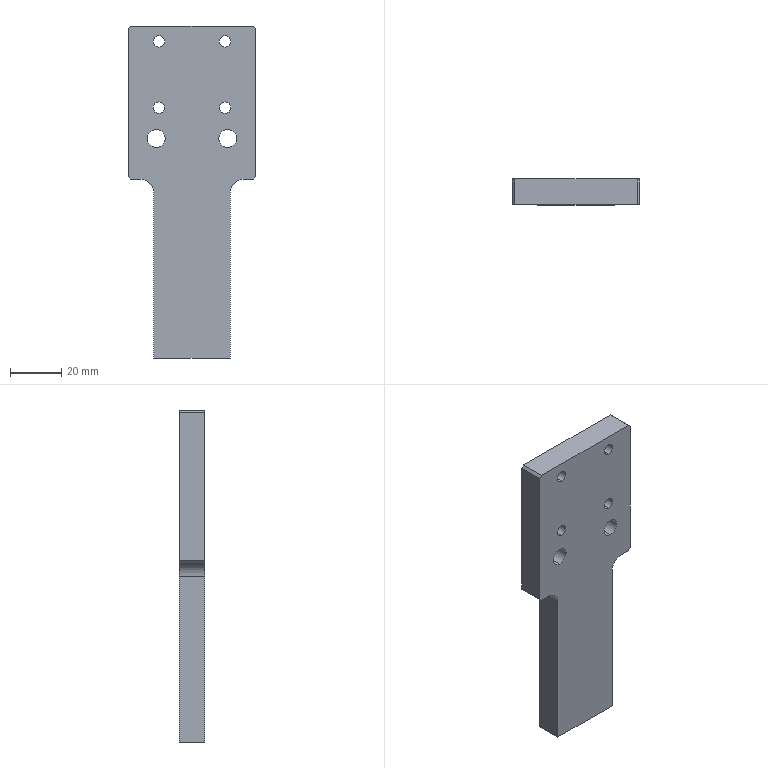Part | 1 solid | 48 faces | box 50 x 10 x 130 mm | volume 48871 mm3 | cylinder 26 | plane 18 | cone 4 | commonest cylinder face diameters 4.5 x8 8 x8 3.3 x4 7 x4 10 x2
STEP:
#1=CARTESIAN_POINT('',(-8.35,0.,-89.9));
#2=VERTEX_POINT('',#1);
#3=CARTESIAN_POINT('',(-11.65,0.,-89.9));
#4=VERTEX_POINT('',#3);
#5=CARTESIAN_POINT('',(-10.,0.,-89.9));
#6=DIRECTION('',(0.,0.,-1.));
#7=DIRECTION('',(-1.,0.,0.));
#8=AXIS2_PLACEMENT_3D('',#5,#6,#7);
#9=CIRCLE('',#8,1.65);
#10=EDGE_CURVE('',#2,#4,#9,.T.);
#11=ORIENTED_EDGE('',*,*,#10,.F.);
#12=CARTESIAN_POINT('',(-8.35,0.,-100.));
#13=VERTEX_POINT('',#12);
#14=CARTESIAN_POINT('',(-8.35,0.,-100.));
#15=DIRECTION('',(0.,0.,-1.));
#16=VECTOR('',#15,1000.);
#17=LINE('',#14,#16);
#18=EDGE_CURVE('',#2,#13,#17,.T.);
#19=ORIENTED_EDGE('',*,*,#18,.T.);
#20=CARTESIAN_POINT('',(-11.65,0.,-100.));
#21=VERTEX_POINT('',#20);
#22=CARTESIAN_POINT('',(-10.,0.,-100.));
#23=DIRECTION('',(0.,0.,-1.));
#24=DIRECTION('',(-1.,0.,0.));
#25=AXIS2_PLACEMENT_3D('',#22,#23,#24);
#26=CIRCLE('',#25,1.65);
#27=EDGE_CURVE('',#13,#21,#26,.T.);
#28=ORIENTED_EDGE('',*,*,#27,.T.);
#29=CARTESIAN_POINT('',(-11.65,0.,-100.));
#30=DIRECTION('',(0.,0.,-1.));
#31=VECTOR('',#30,1000.);
#32=LINE('',#29,#31);
#33=EDGE_CURVE('',#4,#21,#32,.T.);
#34=ORIENTED_EDGE('',*,*,#33,.F.);
#35=EDGE_LOOP('',(#11,#19,#28,#34));
#36=FACE_OUTER_BOUND('',#35,.T.);
#37=CARTESIAN_POINT('',(-10.,0.,-100.));
#38=DIRECTION('',(0.,0.,-1.));
#39=DIRECTION('',(-1.,0.,0.));
#40=AXIS2_PLACEMENT_3D('',#37,#38,#39);
#41=CYLINDRICAL_SURFACE('',#40,1.65);
#42=ADVANCED_FACE('',(#36),#41,.F.);
#43=CARTESIAN_POINT('',(-10.,0.,-88.909));
#44=VERTEX_POINT('',#43);
#45=CARTESIAN_POINT('',(-11.65,0.,-89.9));
#46=DIRECTION('',(-0.8572,0.,-0.515));
#47=VECTOR('',#46,1000.);
#48=LINE('',#45,#47);
#49=EDGE_CURVE('',#44,#4,#48,.T.);
#50=ORIENTED_EDGE('',*,*,#49,.F.);
#51=CARTESIAN_POINT('',(-8.35,0.,-89.9));
#52=DIRECTION('',(0.8572,0.,-0.515));
#53=VECTOR('',#52,1000.);
#54=LINE('',#51,#53);
#55=EDGE_CURVE('',#44,#2,#54,.T.);
#56=ORIENTED_EDGE('',*,*,#55,.T.);
#57=ORIENTED_EDGE('',*,*,#10,.T.);
#58=EDGE_LOOP('',(#50,#56,#57));
#59=FACE_OUTER_BOUND('',#58,.T.);
#60=CARTESIAN_POINT('',(-10.,0.,-89.9));
#61=DIRECTION('',(0.,0.,-1.));
#62=DIRECTION('',(-1.,0.,0.));
#63=AXIS2_PLACEMENT_3D('',#60,#61,#62);
#64=CONICAL_SURFACE('',#63,1.65,1.03);
#65=ADVANCED_FACE('',(#59),#64,.F.);
#66=CARTESIAN_POINT('',(11.65,0.,-89.9));
#67=VERTEX_POINT('',#66);
#68=CARTESIAN_POINT('',(8.35,0.,-89.9));
#69=VERTEX_POINT('',#68);
#70=CARTESIAN_POINT('',(10.,0.,-89.9));
#71=DIRECTION('',(0.,0.,-1.));
#72=DIRECTION('',(-1.,0.,0.));
#73=AXIS2_PLACEMENT_3D('',#70,#71,#72);
#74=CIRCLE('',#73,1.65);
#75=EDGE_CURVE('',#67,#69,#74,.T.);
#76=ORIENTED_EDGE('',*,*,#75,.F.);
#77=CARTESIAN_POINT('',(11.65,0.,-100.));
#78=VERTEX_POINT('',#77);
#79=CARTESIAN_POINT('',(11.65,0.,-100.));
#80=DIRECTION('',(0.,0.,-1.));
#81=VECTOR('',#80,1000.);
#82=LINE('',#79,#81);
#83=EDGE_CURVE('',#67,#78,#82,.T.);
#84=ORIENTED_EDGE('',*,*,#83,.T.);
#85=CARTESIAN_POINT('',(8.35,0.,-100.));
#86=VERTEX_POINT('',#85);
#87=CARTESIAN_POINT('',(10.,0.,-100.));
#88=DIRECTION('',(0.,0.,-1.));
#89=DIRECTION('',(-1.,0.,0.));
#90=AXIS2_PLACEMENT_3D('',#87,#88,#89);
#91=CIRCLE('',#90,1.65);
#92=EDGE_CURVE('',#78,#86,#91,.T.);
#93=ORIENTED_EDGE('',*,*,#92,.T.);
#94=CARTESIAN_POINT('',(8.35,0.,-100.));
#95=DIRECTION('',(0.,0.,-1.));
#96=VECTOR('',#95,1000.);
#97=LINE('',#94,#96);
#98=EDGE_CURVE('',#69,#86,#97,.T.);
#99=ORIENTED_EDGE('',*,*,#98,.F.);
#100=EDGE_LOOP('',(#76,#84,#93,#99));
#101=FACE_OUTER_BOUND('',#100,.T.);
#102=CARTESIAN_POINT('',(10.,0.,-100.));
#103=DIRECTION('',(0.,0.,-1.));
#104=DIRECTION('',(-1.,0.,0.));
#105=AXIS2_PLACEMENT_3D('',#102,#103,#104);
#106=CYLINDRICAL_SURFACE('',#105,1.65);
#107=ADVANCED_FACE('',(#101),#106,.F.);
#108=CARTESIAN_POINT('',(10.,0.,-88.909));
#109=VERTEX_POINT('',#108);
#110=CARTESIAN_POINT('',(8.35,0.,-89.9));
#111=DIRECTION('',(-0.8572,0.,-0.515));
#112=VECTOR('',#111,1000.);
#113=LINE('',#110,#112);
#114=EDGE_CURVE('',#109,#69,#113,.T.);
#115=ORIENTED_EDGE('',*,*,#114,.F.);
#116=CARTESIAN_POINT('',(11.65,0.,-89.9));
#117=DIRECTION('',(0.8572,0.,-0.515));
#118=VECTOR('',#117,1000.);
#119=LINE('',#116,#118);
#120=EDGE_CURVE('',#109,#67,#119,.T.);
#121=ORIENTED_EDGE('',*,*,#120,.T.);
#122=ORIENTED_EDGE('',*,*,#75,.T.);
#123=EDGE_LOOP('',(#115,#121,#122));
#124=FACE_OUTER_BOUND('',#123,.T.);
#125=CARTESIAN_POINT('',(10.,0.,-89.9));
#126=DIRECTION('',(0.,0.,-1.));
#127=DIRECTION('',(-1.,0.,0.));
#128=AXIS2_PLACEMENT_3D('',#125,#126,#127);
#129=CONICAL_SURFACE('',#128,1.65,1.03);
#130=ADVANCED_FACE('',(#124),#129,.F.);
#131=CARTESIAN_POINT('',(-14.,-5.,-17.5));
#132=VERTEX_POINT('',#131);
#133=CARTESIAN_POINT('',(-14.,-5.,-10.5));
#134=VERTEX_POINT('',#133);
#135=CARTESIAN_POINT('',(-14.,-5.,-14.));
#136=DIRECTION('',(0.,1.,0.));
#137=DIRECTION('',(0.,0.,1.));
#138=AXIS2_PLACEMENT_3D('',#135,#136,#137);
#139=CIRCLE('',#138,3.5);
#140=EDGE_CURVE('',#132,#134,#139,.T.);
#141=ORIENTED_EDGE('',*,*,#140,.F.);
#142=CARTESIAN_POINT('',(-14.,5.,-17.5));
#143=VERTEX_POINT('',#142);
#144=CARTESIAN_POINT('',(-14.,5.,-17.5));
#145=DIRECTION('',(0.,1.,0.));
#146=VECTOR('',#145,1000.);
#147=LINE('',#144,#146);
#148=EDGE_CURVE('',#132,#143,#147,.T.);
#149=ORIENTED_EDGE('',*,*,#148,.T.);
#150=CARTESIAN_POINT('',(-14.,5.,-10.5));
#151=VERTEX_POINT('',#150);
#152=CARTESIAN_POINT('',(-14.,5.,-14.));
#153=DIRECTION('',(0.,1.,0.));
#154=DIRECTION('',(0.,0.,1.));
#155=AXIS2_PLACEMENT_3D('',#152,#153,#154);
#156=CIRCLE('',#155,3.5);
#157=EDGE_CURVE('',#143,#151,#156,.T.);
#158=ORIENTED_EDGE('',*,*,#157,.T.);
#159=CARTESIAN_POINT('',(-14.,5.,-10.5));
#160=DIRECTION('',(0.,1.,0.));
#161=VECTOR('',#160,1000.);
#162=LINE('',#159,#161);
#163=EDGE_CURVE('',#134,#151,#162,.T.);
#164=ORIENTED_EDGE('',*,*,#163,.F.);
#165=EDGE_LOOP('',(#141,#149,#158,#164));
#166=FACE_OUTER_BOUND('',#165,.T.);
#167=CARTESIAN_POINT('',(-14.,5.,-14.));
#168=DIRECTION('',(0.,1.,0.));
#169=DIRECTION('',(0.,0.,1.));
#170=AXIS2_PLACEMENT_3D('',#167,#168,#169);
#171=CYLINDRICAL_SURFACE('',#170,3.5);
#172=ADVANCED_FACE('',(#166),#171,.F.);
#173=CARTESIAN_POINT('',(14.,-5.,-17.5));
#174=VERTEX_POINT('',#173);
#175=CARTESIAN_POINT('',(14.,-5.,-10.5));
#176=VERTEX_POINT('',#175);
#177=CARTESIAN_POINT('',(14.,-5.,-14.));
#178=DIRECTION('',(0.,1.,0.));
#179=DIRECTION('',(0.,0.,1.));
#180=AXIS2_PLACEMENT_3D('',#177,#178,#179);
#181=CIRCLE('',#180,3.5);
#182=EDGE_CURVE('',#174,#176,#181,.T.);
#183=ORIENTED_EDGE('',*,*,#182,.F.);
#184=CARTESIAN_POINT('',(14.,5.,-17.5));
#185=VERTEX_POINT('',#184);
#186=CARTESIAN_POINT('',(14.,5.,-17.5));
#187=DIRECTION('',(0.,1.,0.));
#188=VECTOR('',#187,1000.);
#189=LINE('',#186,#188);
#190=EDGE_CURVE('',#174,#185,#189,.T.);
#191=ORIENTED_EDGE('',*,*,#190,.T.);
#192=CARTESIAN_POINT('',(14.,5.,-10.5));
#193=VERTEX_POINT('',#192);
#194=CARTESIAN_POINT('',(14.,5.,-14.));
#195=DIRECTION('',(0.,1.,0.));
#196=DIRECTION('',(0.,0.,1.));
#197=AXIS2_PLACEMENT_3D('',#194,#195,#196);
#198=CIRCLE('',#197,3.5);
#199=EDGE_CURVE('',#185,#193,#198,.T.);
#200=ORIENTED_EDGE('',*,*,#199,.T.);
#201=CARTESIAN_POINT('',(14.,5.,-10.5));
#202=DIRECTION('',(0.,1.,0.));
#203=VECTOR('',#202,1000.);
#204=LINE('',#201,#203);
#205=EDGE_CURVE('',#176,#193,#204,.T.);
#206=ORIENTED_EDGE('',*,*,#205,.F.);
#207=EDGE_LOOP('',(#183,#191,#200,#206));
#208=FACE_OUTER_BOUND('',#207,.T.);
#209=CARTESIAN_POINT('',(14.,5.,-14.));
#210=DIRECTION('',(0.,1.,0.));
#211=DIRECTION('',(0.,0.,1.));
#212=AXIS2_PLACEMENT_3D('',#209,#210,#211);
#213=CYLINDRICAL_SURFACE('',#212,3.5);
#214=ADVANCED_FACE('',(#208),#213,.F.);
#215=CARTESIAN_POINT('',(13.,0.4,20.));
#216=VERTEX_POINT('',#215);
#217=CARTESIAN_POINT('',(13.,0.4,28.));
#218=VERTEX_POINT('',#217);
#219=CARTESIAN_POINT('',(13.,0.4,24.));
#220=DIRECTION('',(0.,1.,0.));
#221=DIRECTION('',(0.,0.,1.));
#222=AXIS2_PLACEMENT_3D('',#219,#220,#221);
#223=CIRCLE('',#222,4.);
#224=EDGE_CURVE('',#216,#218,#223,.T.);
#225=ORIENTED_EDGE('',*,*,#224,.F.);
#226=CARTESIAN_POINT('',(13.,5.,20.));
#227=VERTEX_POINT('',#226);
#228=CARTESIAN_POINT('',(13.,5.,20.));
#229=DIRECTION('',(0.,1.,0.));
#230=VECTOR('',#229,1000.);
#231=LINE('',#228,#230);
#232=EDGE_CURVE('',#216,#227,#231,.T.);
#233=ORIENTED_EDGE('',*,*,#232,.T.);
#234=CARTESIAN_POINT('',(13.,5.,28.));
#235=VERTEX_POINT('',#234);
#236=CARTESIAN_POINT('',(13.,5.,24.));
#237=DIRECTION('',(0.,1.,0.));
#238=DIRECTION('',(0.,0.,1.));
#239=AXIS2_PLACEMENT_3D('',#236,#237,#238);
#240=CIRCLE('',#239,4.);
#241=EDGE_CURVE('',#227,#235,#240,.T.);
#242=ORIENTED_EDGE('',*,*,#241,.T.);
#243=CARTESIAN_POINT('',(13.,5.,28.));
#244=DIRECTION('',(0.,1.,0.));
#245=VECTOR('',#244,1000.);
#246=LINE('',#243,#245);
#247=EDGE_CURVE('',#218,#235,#246,.T.);
#248=ORIENTED_EDGE('',*,*,#247,.F.);
#249=EDGE_LOOP('',(#225,#233,#242,#248));
#250=FACE_OUTER_BOUND('',#249,.T.);
#251=CARTESIAN_POINT('',(13.,5.,24.));
#252=DIRECTION('',(0.,1.,0.));
#253=DIRECTION('',(0.,0.,1.));
#254=AXIS2_PLACEMENT_3D('',#251,#252,#253);
#255=CYLINDRICAL_SURFACE('',#254,4.);
#256=ADVANCED_FACE('',(#250),#255,.F.);
#257=CARTESIAN_POINT('',(13.,-5.,21.75));
#258=VERTEX_POINT('',#257);
#259=CARTESIAN_POINT('',(13.,-5.,26.25));
#260=VERTEX_POINT('',#259);
#261=CARTESIAN_POINT('',(13.,-5.,24.));
#262=DIRECTION('',(0.,1.,0.));
#263=DIRECTION('',(0.,0.,1.));
#264=AXIS2_PLACEMENT_3D('',#261,#262,#263);
#265=CIRCLE('',#264,2.25);
#266=EDGE_CURVE('',#258,#260,#265,.T.);
#267=ORIENTED_EDGE('',*,*,#266,.F.);
#268=CARTESIAN_POINT('',(13.,0.4,21.75));
#269=VERTEX_POINT('',#268);
#270=CARTESIAN_POINT('',(13.,5.,21.75));
#271=DIRECTION('',(0.,1.,0.));
#272=VECTOR('',#271,1000.);
#273=LINE('',#270,#272);
#274=EDGE_CURVE('',#258,#269,#273,.T.);
#275=ORIENTED_EDGE('',*,*,#274,.T.);
#276=CARTESIAN_POINT('',(13.,0.4,26.25));
#277=VERTEX_POINT('',#276);
#278=CARTESIAN_POINT('',(13.,0.4,24.));
#279=DIRECTION('',(0.,1.,0.));
#280=DIRECTION('',(0.,0.,1.));
#281=AXIS2_PLACEMENT_3D('',#278,#279,#280);
#282=CIRCLE('',#281,2.25);
#283=EDGE_CURVE('',#269,#277,#282,.T.);
#284=ORIENTED_EDGE('',*,*,#283,.T.);
#285=CARTESIAN_POINT('',(13.,5.,26.25));
#286=DIRECTION('',(0.,1.,0.));
#287=VECTOR('',#286,1000.);
#288=LINE('',#285,#287);
#289=EDGE_CURVE('',#260,#277,#288,.T.);
#290=ORIENTED_EDGE('',*,*,#289,.F.);
#291=EDGE_LOOP('',(#267,#275,#284,#290));
#292=FACE_OUTER_BOUND('',#291,.T.);
#293=CARTESIAN_POINT('',(13.,5.,24.));
#294=DIRECTION('',(0.,1.,0.));
#295=DIRECTION('',(0.,0.,1.));
#296=AXIS2_PLACEMENT_3D('',#293,#294,#295);
#297=CYLINDRICAL_SURFACE('',#296,2.25);
#298=ADVANCED_FACE('',(#292),#297,.F.);
#299=CARTESIAN_POINT('',(13.,0.4,-6.));
#300=VERTEX_POINT('',#299);
#301=CARTESIAN_POINT('',(13.,0.4,2.));
#302=VERTEX_POINT('',#301);
#303=CARTESIAN_POINT('',(13.,0.4,-2.));
#304=DIRECTION('',(0.,1.,0.));
#305=DIRECTION('',(0.,0.,1.));
#306=AXIS2_PLACEMENT_3D('',#303,#304,#305);
#307=CIRCLE('',#306,4.);
#308=EDGE_CURVE('',#300,#302,#307,.T.);
#309=ORIENTED_EDGE('',*,*,#308,.F.);
#310=CARTESIAN_POINT('',(13.,5.,-6.));
#311=VERTEX_POINT('',#310);
#312=CARTESIAN_POINT('',(13.,5.,-6.));
#313=DIRECTION('',(0.,1.,0.));
#314=VECTOR('',#313,1000.);
#315=LINE('',#312,#314);
#316=EDGE_CURVE('',#300,#311,#315,.T.);
#317=ORIENTED_EDGE('',*,*,#316,.T.);
#318=CARTESIAN_POINT('',(13.,5.,2.));
#319=VERTEX_POINT('',#318);
#320=CARTESIAN_POINT('',(13.,5.,-2.));
#321=DIRECTION('',(0.,1.,0.));
#322=DIRECTION('',(0.,0.,1.));
#323=AXIS2_PLACEMENT_3D('',#320,#321,#322);
#324=CIRCLE('',#323,4.);
#325=EDGE_CURVE('',#311,#319,#324,.T.);
#326=ORIENTED_EDGE('',*,*,#325,.T.);
#327=CARTESIAN_POINT('',(13.,5.,2.));
#328=DIRECTION('',(0.,1.,0.));
#329=VECTOR('',#328,1000.);
#330=LINE('',#327,#329);
#331=EDGE_CURVE('',#302,#319,#330,.T.);
#332=ORIENTED_EDGE('',*,*,#331,.F.);
#333=EDGE_LOOP('',(#309,#317,#326,#332));
#334=FACE_OUTER_BOUND('',#333,.T.);
#335=CARTESIAN_POINT('',(13.,5.,-2.));
#336=DIRECTION('',(0.,1.,0.));
#337=DIRECTION('',(0.,0.,1.));
#338=AXIS2_PLACEMENT_3D('',#335,#336,#337);
#339=CYLINDRICAL_SURFACE('',#338,4.);
#340=ADVANCED_FACE('',(#334),#339,.F.);
#341=CARTESIAN_POINT('',(13.,-5.,-4.25));
#342=VERTEX_POINT('',#341);
#343=CARTESIAN_POINT('',(13.,-5.,0.25));
#344=VERTEX_POINT('',#343);
#345=CARTESIAN_POINT('',(13.,-5.,-2.));
#346=DIRECTION('',(0.,1.,0.));
#347=DIRECTION('',(0.,0.,1.));
#348=AXIS2_PLACEMENT_3D('',#345,#346,#347);
#349=CIRCLE('',#348,2.25);
#350=EDGE_CURVE('',#342,#344,#349,.T.);
#351=ORIENTED_EDGE('',*,*,#350,.F.);
#352=CARTESIAN_POINT('',(13.,0.4,-4.25));
#353=VERTEX_POINT('',#352);
#354=CARTESIAN_POINT('',(13.,5.,-4.25));
#355=DIRECTION('',(0.,1.,0.));
#356=VECTOR('',#355,1000.);
#357=LINE('',#354,#356);
#358=EDGE_CURVE('',#342,#353,#357,.T.);
#359=ORIENTED_EDGE('',*,*,#358,.T.);
#360=CARTESIAN_POINT('',(13.,0.4,0.25));
#361=VERTEX_POINT('',#360);
#362=CARTESIAN_POINT('',(13.,0.4,-2.));
#363=DIRECTION('',(0.,1.,0.));
#364=DIRECTION('',(0.,0.,1.));
#365=AXIS2_PLACEMENT_3D('',#362,#363,#364);
#366=CIRCLE('',#365,2.25);
#367=EDGE_CURVE('',#353,#361,#366,.T.);
#368=ORIENTED_EDGE('',*,*,#367,.T.);
#369=CARTESIAN_POINT('',(13.,5.,0.25));
#370=DIRECTION('',(0.,1.,0.));
#371=VECTOR('',#370,1000.);
#372=LINE('',#369,#371);
#373=EDGE_CURVE('',#344,#361,#372,.T.);
#374=ORIENTED_EDGE('',*,*,#373,.F.);
#375=EDGE_LOOP('',(#351,#359,#368,#374));
#376=FACE_OUTER_BOUND('',#375,.T.);
#377=CARTESIAN_POINT('',(13.,5.,-2.));
#378=DIRECTION('',(0.,1.,0.));
#379=DIRECTION('',(0.,0.,1.));
#380=AXIS2_PLACEMENT_3D('',#377,#378,#379);
#381=CYLINDRICAL_SURFACE('',#380,2.25);
#382=ADVANCED_FACE('',(#376),#381,.F.);
#383=CARTESIAN_POINT('',(-13.,0.4,-6.));
#384=VERTEX_POINT('',#383);
#385=CARTESIAN_POINT('',(-13.,0.4,2.));
#386=VERTEX_POINT('',#385);
#387=CARTESIAN_POINT('',(-13.,0.4,-2.));
#388=DIRECTION('',(0.,1.,0.));
#389=DIRECTION('',(0.,0.,1.));
#390=AXIS2_PLACEMENT_3D('',#387,#388,#389);
#391=CIRCLE('',#390,4.);
#392=EDGE_CURVE('',#384,#386,#391,.T.);
#393=ORIENTED_EDGE('',*,*,#392,.F.);
#394=CARTESIAN_POINT('',(-13.,5.,-6.));
#395=VERTEX_POINT('',#394);
#396=CARTESIAN_POINT('',(-13.,5.,-6.));
#397=DIRECTION('',(0.,1.,0.));
#398=VECTOR('',#397,1000.);
#399=LINE('',#396,#398);
#400=EDGE_CURVE('',#384,#395,#399,.T.);
#401=ORIENTED_EDGE('',*,*,#400,.T.);
#402=CARTESIAN_POINT('',(-13.,5.,2.));
#403=VERTEX_POINT('',#402);
#404=CARTESIAN_POINT('',(-13.,5.,-2.));
#405=DIRECTION('',(0.,1.,0.));
#406=DIRECTION('',(0.,0.,1.));
#407=AXIS2_PLACEMENT_3D('',#404,#405,#406);
#408=CIRCLE('',#407,4.);
#409=EDGE_CURVE('',#395,#403,#408,.T.);
#410=ORIENTED_EDGE('',*,*,#409,.T.);
#411=CARTESIAN_POINT('',(-13.,5.,2.));
#412=DIRECTION('',(0.,1.,0.));
#413=VECTOR('',#412,1000.);
#414=LINE('',#411,#413);
#415=EDGE_CURVE('',#386,#403,#414,.T.);
#416=ORIENTED_EDGE('',*,*,#415,.F.);
#417=EDGE_LOOP('',(#393,#401,#410,#416));
#418=FACE_OUTER_BOUND('',#417,.T.);
#419=CARTESIAN_POINT('',(-13.,5.,-2.));
#420=DIRECTION('',(0.,1.,0.));
#421=DIRECTION('',(0.,0.,1.));
#422=AXIS2_PLACEMENT_3D('',#419,#420,#421);
#423=CYLINDRICAL_SURFACE('',#422,4.);
#424=ADVANCED_FACE('',(#418),#423,.F.);
#425=CARTESIAN_POINT('',(-13.,-5.,-4.25));
#426=VERTEX_POINT('',#425);
#427=CARTESIAN_POINT('',(-13.,-5.,0.25));
#428=VERTEX_POINT('',#427);
#429=CARTESIAN_POINT('',(-13.,-5.,-2.));
#430=DIRECTION('',(0.,1.,0.));
#431=DIRECTION('',(0.,0.,1.));
#432=AXIS2_PLACEMENT_3D('',#429,#430,#431);
#433=CIRCLE('',#432,2.25);
#434=EDGE_CURVE('',#426,#428,#433,.T.);
#435=ORIENTED_EDGE('',*,*,#434,.F.);
#436=CARTESIAN_POINT('',(-13.,0.4,-4.25));
#437=VERTEX_POINT('',#436);
#438=CARTESIAN_POINT('',(-13.,5.,-4.25));
#439=DIRECTION('',(0.,1.,0.));
#440=VECTOR('',#439,1000.);
#441=LINE('',#438,#440);
#442=EDGE_CURVE('',#426,#437,#441,.T.);
#443=ORIENTED_EDGE('',*,*,#442,.T.);
#444=CARTESIAN_POINT('',(-13.,0.4,0.25));
#445=VERTEX_POINT('',#444);
#446=CARTESIAN_POINT('',(-13.,0.4,-2.));
#447=DIRECTION('',(0.,1.,0.));
#448=DIRECTION('',(0.,0.,1.));
#449=AXIS2_PLACEMENT_3D('',#446,#447,#448);
#450=CIRCLE('',#449,2.25);
#451=EDGE_CURVE('',#437,#445,#450,.T.);
#452=ORIENTED_EDGE('',*,*,#451,.T.);
#453=CARTESIAN_POINT('',(-13.,5.,0.25));
#454=DIRECTION('',(0.,1.,0.));
#455=VECTOR('',#454,1000.);
#456=LINE('',#453,#455);
#457=EDGE_CURVE('',#428,#445,#456,.T.);
#458=ORIENTED_EDGE('',*,*,#457,.F.);
#459=EDGE_LOOP('',(#435,#443,#452,#458));
#460=FACE_OUTER_BOUND('',#459,.T.);
#461=CARTESIAN_POINT('',(-13.,5.,-2.));
#462=DIRECTION('',(0.,1.,0.));
#463=DIRECTION('',(0.,0.,1.));
#464=AXIS2_PLACEMENT_3D('',#461,#462,#463);
#465=CYLINDRICAL_SURFACE('',#464,2.25);
#466=ADVANCED_FACE('',(#460),#465,.F.);
#467=CARTESIAN_POINT('',(-13.,0.4,20.));
#468=VERTEX_POINT('',#467);
#469=CARTESIAN_POINT('',(-13.,0.4,28.));
#470=VERTEX_POINT('',#469);
#471=CARTESIAN_POINT('',(-13.,0.4,24.));
#472=DIRECTION('',(0.,1.,0.));
#473=DIRECTION('',(0.,0.,1.));
#474=AXIS2_PLACEMENT_3D('',#471,#472,#473);
#475=CIRCLE('',#474,4.);
#476=EDGE_CURVE('',#468,#470,#475,.T.);
#477=ORIENTED_EDGE('',*,*,#476,.F.);
#478=CARTESIAN_POINT('',(-13.,5.,20.));
#479=VERTEX_POINT('',#478);
#480=CARTESIAN_POINT('',(-13.,5.,20.));
#481=DIRECTION('',(0.,1.,0.));
#482=VECTOR('',#481,1000.);
#483=LINE('',#480,#482);
#484=EDGE_CURVE('',#468,#479,#483,.T.);
#485=ORIENTED_EDGE('',*,*,#484,.T.);
#486=CARTESIAN_POINT('',(-13.,5.,28.));
#487=VERTEX_POINT('',#486);
#488=CARTESIAN_POINT('',(-13.,5.,24.));
#489=DIRECTION('',(0.,1.,0.));
#490=DIRECTION('',(0.,0.,1.));
#491=AXIS2_PLACEMENT_3D('',#488,#489,#490);
#492=CIRCLE('',#491,4.);
#493=EDGE_CURVE('',#479,#487,#492,.T.);
#494=ORIENTED_EDGE('',*,*,#493,.T.);
#495=CARTESIAN_POINT('',(-13.,5.,28.));
#496=DIRECTION('',(0.,1.,0.));
#497=VECTOR('',#496,1000.);
#498=LINE('',#495,#497);
#499=EDGE_CURVE('',#470,#487,#498,.T.);
#500=ORIENTED_EDGE('',*,*,#499,.F.);
#501=EDGE_LOOP('',(#477,#485,#494,#500));
#502=FACE_OUTER_BOUND('',#501,.T.);
#503=CARTESIAN_POINT('',(-13.,5.,24.));
#504=DIRECTION('',(0.,1.,0.));
#505=DIRECTION('',(0.,0.,1.));
#506=AXIS2_PLACEMENT_3D('',#503,#504,#505);
#507=CYLINDRICAL_SURFACE('',#506,4.);
#508=ADVANCED_FACE('',(#502),#507,.F.);
#509=CARTESIAN_POINT('',(-13.,-5.,21.75));
#510=VERTEX_POINT('',#509);
#511=CARTESIAN_POINT('',(-13.,-5.,26.25));
#512=VERTEX_POINT('',#511);
#513=CARTESIAN_POINT('',(-13.,-5.,24.));
#514=DIRECTION('',(0.,1.,0.));
#515=DIRECTION('',(0.,0.,1.));
#516=AXIS2_PLACEMENT_3D('',#513,#514,#515);
#517=CIRCLE('',#516,2.25);
#518=EDGE_CURVE('',#510,#512,#517,.T.);
#519=ORIENTED_EDGE('',*,*,#518,.F.);
#520=CARTESIAN_POINT('',(-13.,0.4,21.75));
#521=VERTEX_POINT('',#520);
#522=CARTESIAN_POINT('',(-13.,5.,21.75));
#523=DIRECTION('',(0.,1.,0.));
#524=VECTOR('',#523,1000.);
#525=LINE('',#522,#524);
#526=EDGE_CURVE('',#510,#521,#525,.T.);
#527=ORIENTED_EDGE('',*,*,#526,.T.);
#528=CARTESIAN_POINT('',(-13.,0.4,26.25));
#529=VERTEX_POINT('',#528);
#530=CARTESIAN_POINT('',(-13.,0.4,24.));
#531=DIRECTION('',(0.,1.,0.));
#532=DIRECTION('',(0.,0.,1.));
#533=AXIS2_PLACEMENT_3D('',#530,#531,#532);
#534=CIRCLE('',#533,2.25);
#535=EDGE_CURVE('',#521,#529,#534,.T.);
#536=ORIENTED_EDGE('',*,*,#535,.T.);
#537=CARTESIAN_POINT('',(-13.,5.,26.25));
#538=DIRECTION('',(0.,1.,0.));
#539=VECTOR('',#538,1000.);
#540=LINE('',#537,#539);
#541=EDGE_CURVE('',#512,#529,#540,.T.);
#542=ORIENTED_EDGE('',*,*,#541,.F.);
#543=EDGE_LOOP('',(#519,#527,#536,#542));
#544=FACE_OUTER_BOUND('',#543,.T.);
#545=CARTESIAN_POINT('',(-13.,5.,24.));
#546=DIRECTION('',(0.,1.,0.));
#547=DIRECTION('',(0.,0.,1.));
#548=AXIS2_PLACEMENT_3D('',#545,#546,#547);
#549=CYLINDRICAL_SURFACE('',#548,2.25);
#550=ADVANCED_FACE('',(#544),#549,.F.);
#551=CARTESIAN_POINT('',(-20.,5.,-30.));
#552=VERTEX_POINT('',#551);
#553=CARTESIAN_POINT('',(-24.,5.,-30.));
#554=VERTEX_POINT('',#553);
#555=CARTESIAN_POINT('',(-25.,5.,-30.));
#556=DIRECTION('',(-1.,0.,0.));
#557=VECTOR('',#556,1000.);
#558=LINE('',#555,#557);
#559=EDGE_CURVE('',#552,#554,#558,.T.);
#560=ORIENTED_EDGE('',*,*,#559,.F.);
#561=CARTESIAN_POINT('',(-20.,-5.,-30.));
#562=VERTEX_POINT('',#561);
#563=CARTESIAN_POINT('',(-20.,5.,-30.));
#564=DIRECTION('',(0.,-1.,0.));
#565=VECTOR('',#564,1000.);
#566=LINE('',#563,#565);
#567=EDGE_CURVE('',#552,#562,#566,.T.);
#568=ORIENTED_EDGE('',*,*,#567,.T.);
#569=CARTESIAN_POINT('',(-24.,-5.,-30.));
#570=VERTEX_POINT('',#569);
#571=CARTESIAN_POINT('',(-25.,-5.,-30.));
#572=DIRECTION('',(-1.,0.,0.));
#573=VECTOR('',#572,1000.);
#574=LINE('',#571,#573);
#575=EDGE_CURVE('',#562,#570,#574,.T.);
#576=ORIENTED_EDGE('',*,*,#575,.T.);
#577=CARTESIAN_POINT('',(-24.,5.,-30.));
#578=DIRECTION('',(0.,1.,0.));
#579=VECTOR('',#578,1000.);
#580=LINE('',#577,#579);
#581=EDGE_CURVE('',#570,#554,#580,.T.);
#582=ORIENTED_EDGE('',*,*,#581,.T.);
#583=EDGE_LOOP('',(#560,#568,#576,#582));
#584=FACE_OUTER_BOUND('',#583,.T.);
#585=CARTESIAN_POINT('',(-25.,5.,-30.));
#586=DIRECTION('',(0.,0.,1.));
#587=DIRECTION('',(1.,0.,0.));
#588=AXIS2_PLACEMENT_3D('',#585,#586,#587);
#589=PLANE('',#588);
#590=ADVANCED_FACE('',(#584),#589,.F.);
#591=CARTESIAN_POINT('',(25.,-5.,29.));
#592=VERTEX_POINT('',#591);
#593=CARTESIAN_POINT('',(25.,-5.,-29.));
#594=VERTEX_POINT('',#593);
#595=CARTESIAN_POINT('',(25.,-5.,30.));
#596=DIRECTION('',(0.,0.,-1.));
#597=VECTOR('',#596,1000.);
#598=LINE('',#595,#597);
#599=EDGE_CURVE('',#592,#594,#598,.T.);
#600=ORIENTED_EDGE('',*,*,#599,.T.);
#601=CARTESIAN_POINT('',(25.,5.,-29.));
#602=VERTEX_POINT('',#601);
#603=CARTESIAN_POINT('',(25.,5.,-29.));
#604=DIRECTION('',(0.,1.,0.));
#605=VECTOR('',#604,1000.);
#606=LINE('',#603,#605);
#607=EDGE_CURVE('',#594,#602,#606,.T.);
#608=ORIENTED_EDGE('',*,*,#607,.T.);
#609=CARTESIAN_POINT('',(25.,5.,29.));
#610=VERTEX_POINT('',#609);
#611=CARTESIAN_POINT('',(25.,5.,30.));
#612=DIRECTION('',(0.,0.,-1.));
#613=VECTOR('',#612,1000.);
#614=LINE('',#611,#613);
#615=EDGE_CURVE('',#610,#602,#614,.T.);
#616=ORIENTED_EDGE('',*,*,#615,.F.);
#617=CARTESIAN_POINT('',(25.,5.,29.));
#618=DIRECTION('',(0.,-1.,0.));
#619=VECTOR('',#618,1000.);
#620=LINE('',#617,#619);
#621=EDGE_CURVE('',#610,#592,#620,.T.);
#622=ORIENTED_EDGE('',*,*,#621,.T.);
#623=EDGE_LOOP('',(#600,#608,#616,#622));
#624=FACE_OUTER_BOUND('',#623,.T.);
#625=CARTESIAN_POINT('',(25.,5.,30.));
#626=DIRECTION('',(-1.,0.,0.));
#627=DIRECTION('',(0.,0.,1.));
#628=AXIS2_PLACEMENT_3D('',#625,#626,#627);
#629=PLANE('',#628);
#630=ADVANCED_FACE('',(#624),#629,.F.);
#631=CARTESIAN_POINT('',(24.,-5.,-30.));
#632=VERTEX_POINT('',#631);
#633=CARTESIAN_POINT('',(20.,-5.,-30.));
#634=VERTEX_POINT('',#633);
#635=CARTESIAN_POINT('',(-25.,-5.,-30.));
#636=DIRECTION('',(-1.,0.,0.));
#637=VECTOR('',#636,1000.);
#638=LINE('',#635,#637);
#639=EDGE_CURVE('',#632,#634,#638,.T.);
#640=ORIENTED_EDGE('',*,*,#639,.T.);
#641=CARTESIAN_POINT('',(20.,5.,-30.));
#642=VERTEX_POINT('',#641);
#643=CARTESIAN_POINT('',(20.,5.,-30.));
#644=DIRECTION('',(0.,1.,0.));
#645=VECTOR('',#644,1000.);
#646=LINE('',#643,#645);
#647=EDGE_CURVE('',#634,#642,#646,.T.);
#648=ORIENTED_EDGE('',*,*,#647,.T.);
#649=CARTESIAN_POINT('',(24.,5.,-30.));
#650=VERTEX_POINT('',#649);
#651=CARTESIAN_POINT('',(-25.,5.,-30.));
#652=DIRECTION('',(-1.,0.,0.));
#653=VECTOR('',#652,1000.);
#654=LINE('',#651,#653);
#655=EDGE_CURVE('',#650,#642,#654,.T.);
#656=ORIENTED_EDGE('',*,*,#655,.F.);
#657=CARTESIAN_POINT('',(24.,5.,-30.));
#658=DIRECTION('',(0.,-1.,0.));
#659=VECTOR('',#658,1000.);
#660=LINE('',#657,#659);
#661=EDGE_CURVE('',#650,#632,#660,.T.);
#662=ORIENTED_EDGE('',*,*,#661,.T.);
#663=EDGE_LOOP('',(#640,#648,#656,#662));
#664=FACE_OUTER_BOUND('',#663,.T.);
#665=CARTESIAN_POINT('',(-25.,5.,-30.));
#666=DIRECTION('',(0.,0.,1.));
#667=DIRECTION('',(1.,0.,0.));
#668=AXIS2_PLACEMENT_3D('',#665,#666,#667);
#669=PLANE('',#668);
#670=ADVANCED_FACE('',(#664),#669,.F.);
#671=CARTESIAN_POINT('',(-25.,5.,-29.));
#672=VERTEX_POINT('',#671);
#673=CARTESIAN_POINT('',(-25.,5.,29.));
#674=VERTEX_POINT('',#673);
#675=CARTESIAN_POINT('',(-25.,5.,30.));
#676=DIRECTION('',(0.,0.,1.));
#677=VECTOR('',#676,1000.);
#678=LINE('',#675,#677);
#679=EDGE_CURVE('',#672,#674,#678,.T.);
#680=ORIENTED_EDGE('',*,*,#679,.F.);
#681=CARTESIAN_POINT('',(-25.,-5.,-29.));
#682=VERTEX_POINT('',#681);
#683=CARTESIAN_POINT('',(-25.,5.,-29.));
#684=DIRECTION('',(0.,-1.,0.));
#685=VECTOR('',#684,1000.);
#686=LINE('',#683,#685);
#687=EDGE_CURVE('',#672,#682,#686,.T.);
#688=ORIENTED_EDGE('',*,*,#687,.T.);
#689=CARTESIAN_POINT('',(-25.,-5.,29.));
#690=VERTEX_POINT('',#689);
#691=CARTESIAN_POINT('',(-25.,-5.,30.));
#692=DIRECTION('',(0.,0.,1.));
#693=VECTOR('',#692,1000.);
#694=LINE('',#691,#693);
#695=EDGE_CURVE('',#682,#690,#694,.T.);
#696=ORIENTED_EDGE('',*,*,#695,.T.);
#697=CARTESIAN_POINT('',(-25.,5.,29.));
#698=DIRECTION('',(0.,1.,0.));
#699=VECTOR('',#698,1000.);
#700=LINE('',#697,#699);
#701=EDGE_CURVE('',#690,#674,#700,.T.);
#702=ORIENTED_EDGE('',*,*,#701,.T.);
#703=EDGE_LOOP('',(#680,#688,#696,#702));
#704=FACE_OUTER_BOUND('',#703,.T.);
#705=CARTESIAN_POINT('',(-25.,5.,30.));
#706=DIRECTION('',(1.,0.,0.));
#707=DIRECTION('',(0.,0.,-1.));
#708=AXIS2_PLACEMENT_3D('',#705,#706,#707);
#709=PLANE('',#708);
#710=ADVANCED_FACE('',(#704),#709,.F.);
#711=CARTESIAN_POINT('',(-24.,-5.,30.));
#712=VERTEX_POINT('',#711);
#713=CARTESIAN_POINT('',(24.,-5.,30.));
#714=VERTEX_POINT('',#713);
#715=CARTESIAN_POINT('',(-25.,-5.,30.));
#716=DIRECTION('',(1.,0.,0.));
#717=VECTOR('',#716,1000.);
#718=LINE('',#715,#717);
#719=EDGE_CURVE('',#712,#714,#718,.T.);
#720=ORIENTED_EDGE('',*,*,#719,.T.);
#721=CARTESIAN_POINT('',(24.,5.,30.));
#722=VERTEX_POINT('',#721);
#723=CARTESIAN_POINT('',(24.,5.,30.));
#724=DIRECTION('',(0.,1.,0.));
#725=VECTOR('',#724,1000.);
#726=LINE('',#723,#725);
#727=EDGE_CURVE('',#714,#722,#726,.T.);
#728=ORIENTED_EDGE('',*,*,#727,.T.);
#729=CARTESIAN_POINT('',(-24.,5.,30.));
#730=VERTEX_POINT('',#729);
#731=CARTESIAN_POINT('',(-25.,5.,30.));
#732=DIRECTION('',(1.,0.,0.));
#733=VECTOR('',#732,1000.);
#734=LINE('',#731,#733);
#735=EDGE_CURVE('',#730,#722,#734,.T.);
#736=ORIENTED_EDGE('',*,*,#735,.F.);
#737=CARTESIAN_POINT('',(-24.,5.,30.));
#738=DIRECTION('',(0.,-1.,0.));
#739=VECTOR('',#738,1000.);
#740=LINE('',#737,#739);
#741=EDGE_CURVE('',#730,#712,#740,.T.);
#742=ORIENTED_EDGE('',*,*,#741,.T.);
#743=EDGE_LOOP('',(#720,#728,#736,#742));
#744=FACE_OUTER_BOUND('',#743,.T.);
#745=CARTESIAN_POINT('',(-25.,5.,30.));
#746=DIRECTION('',(0.,0.,-1.));
#747=DIRECTION('',(-1.,0.,0.));
#748=AXIS2_PLACEMENT_3D('',#745,#746,#747);
#749=PLANE('',#748);
#750=ADVANCED_FACE('',(#744),#749,.F.);
#751=CARTESIAN_POINT('',(-14.,5.,-14.));
#752=DIRECTION('',(0.,1.,0.));
#753=DIRECTION('',(0.,0.,1.));
#754=AXIS2_PLACEMENT_3D('',#751,#752,#753);
#755=CIRCLE('',#754,3.5);
#756=EDGE_CURVE('',#151,#143,#755,.T.);
#757=ORIENTED_EDGE('',*,*,#756,.F.);
#758=ORIENTED_EDGE('',*,*,#157,.F.);
#759=EDGE_LOOP('',(#757,#758));
#760=FACE_BOUND('',#759,.T.);
#761=CARTESIAN_POINT('',(14.,5.,-14.));
#762=DIRECTION('',(0.,1.,0.));
#763=DIRECTION('',(0.,0.,1.));
#764=AXIS2_PLACEMENT_3D('',#761,#762,#763);
#765=CIRCLE('',#764,3.5);
#766=EDGE_CURVE('',#193,#185,#765,.T.);
#767=ORIENTED_EDGE('',*,*,#766,.F.);
#768=ORIENTED_EDGE('',*,*,#199,.F.);
#769=EDGE_LOOP('',(#767,#768));
#770=FACE_BOUND('',#769,.T.);
#771=CARTESIAN_POINT('',(13.,5.,24.));
#772=DIRECTION('',(0.,1.,0.));
#773=DIRECTION('',(0.,0.,1.));
#774=AXIS2_PLACEMENT_3D('',#771,#772,#773);
#775=CIRCLE('',#774,4.);
#776=EDGE_CURVE('',#235,#227,#775,.T.);
#777=ORIENTED_EDGE('',*,*,#776,.F.);
#778=ORIENTED_EDGE('',*,*,#241,.F.);
#779=EDGE_LOOP('',(#777,#778));
#780=FACE_BOUND('',#779,.T.);
#781=CARTESIAN_POINT('',(13.,5.,-2.));
#782=DIRECTION('',(0.,1.,0.));
#783=DIRECTION('',(0.,0.,1.));
#784=AXIS2_PLACEMENT_3D('',#781,#782,#783);
#785=CIRCLE('',#784,4.);
#786=EDGE_CURVE('',#319,#311,#785,.T.);
#787=ORIENTED_EDGE('',*,*,#786,.F.);
#788=ORIENTED_EDGE('',*,*,#325,.F.);
#789=EDGE_LOOP('',(#787,#788));
#790=FACE_BOUND('',#789,.T.);
#791=CARTESIAN_POINT('',(-13.,5.,-2.));
#792=DIRECTION('',(0.,1.,0.));
#793=DIRECTION('',(0.,0.,1.));
#794=AXIS2_PLACEMENT_3D('',#791,#792,#793);
#795=CIRCLE('',#794,4.);
#796=EDGE_CURVE('',#403,#395,#795,.T.);
#797=ORIENTED_EDGE('',*,*,#796,.F.);
#798=ORIENTED_EDGE('',*,*,#409,.F.);
#799=EDGE_LOOP('',(#797,#798));
#800=FACE_BOUND('',#799,.T.);
#801=CARTESIAN_POINT('',(-13.,5.,24.));
#802=DIRECTION('',(0.,1.,0.));
#803=DIRECTION('',(0.,0.,1.));
#804=AXIS2_PLACEMENT_3D('',#801,#802,#803);
#805=CIRCLE('',#804,4.);
#806=EDGE_CURVE('',#487,#479,#805,.T.);
#807=ORIENTED_EDGE('',*,*,#806,.F.);
#808=ORIENTED_EDGE('',*,*,#493,.F.);
#809=EDGE_LOOP('',(#807,#808));
#810=FACE_BOUND('',#809,.T.);
#811=ORIENTED_EDGE('',*,*,#615,.T.);
#812=CARTESIAN_POINT('',(24.,5.,-30.));
#813=DIRECTION('',(-0.7071,0.,-0.7071));
#814=VECTOR('',#813,1000.);
#815=LINE('',#812,#814);
#816=EDGE_CURVE('',#602,#650,#815,.T.);
#817=ORIENTED_EDGE('',*,*,#816,.T.);
#818=ORIENTED_EDGE('',*,*,#655,.T.);
#819=CARTESIAN_POINT('',(15.,5.,-35.));
#820=VERTEX_POINT('',#819);
#821=CARTESIAN_POINT('',(20.,5.,-35.));
#822=DIRECTION('',(0.,-1.,0.));
#823=DIRECTION('',(0.,0.,-1.));
#824=AXIS2_PLACEMENT_3D('',#821,#822,#823);
#825=CIRCLE('',#824,5.);
#826=EDGE_CURVE('',#642,#820,#825,.T.);
#827=ORIENTED_EDGE('',*,*,#826,.T.);
#828=CARTESIAN_POINT('',(15.,5.,-100.));
#829=VERTEX_POINT('',#828);
#830=CARTESIAN_POINT('',(15.,5.,-30.));
#831=DIRECTION('',(0.,0.,-1.));
#832=VECTOR('',#831,1000.);
#833=LINE('',#830,#832);
#834=EDGE_CURVE('',#820,#829,#833,.T.);
#835=ORIENTED_EDGE('',*,*,#834,.T.);
#836=CARTESIAN_POINT('',(-15.,5.,-100.));
#837=VERTEX_POINT('',#836);
#838=CARTESIAN_POINT('',(15.,5.,-100.));
#839=DIRECTION('',(-1.,0.,0.));
#840=VECTOR('',#839,1000.);
#841=LINE('',#838,#840);
#842=EDGE_CURVE('',#829,#837,#841,.T.);
#843=ORIENTED_EDGE('',*,*,#842,.T.);
#844=CARTESIAN_POINT('',(-15.,5.,-35.));
#845=VERTEX_POINT('',#844);
#846=CARTESIAN_POINT('',(-15.,5.,-30.));
#847=DIRECTION('',(0.,0.,1.));
#848=VECTOR('',#847,1000.);
#849=LINE('',#846,#848);
#850=EDGE_CURVE('',#837,#845,#849,.T.);
#851=ORIENTED_EDGE('',*,*,#850,.T.);
#852=CARTESIAN_POINT('',(-20.,5.,-35.));
#853=DIRECTION('',(0.,-1.,0.));
#854=DIRECTION('',(0.,0.,-1.));
#855=AXIS2_PLACEMENT_3D('',#852,#853,#854);
#856=CIRCLE('',#855,5.);
#857=EDGE_CURVE('',#845,#552,#856,.T.);
#858=ORIENTED_EDGE('',*,*,#857,.T.);
#859=ORIENTED_EDGE('',*,*,#559,.T.);
#860=CARTESIAN_POINT('',(-25.,5.,-29.));
#861=DIRECTION('',(-0.7071,0.,0.7071));
#862=VECTOR('',#861,1000.);
#863=LINE('',#860,#862);
#864=EDGE_CURVE('',#554,#672,#863,.T.);
#865=ORIENTED_EDGE('',*,*,#864,.T.);
#866=ORIENTED_EDGE('',*,*,#679,.T.);
#867=CARTESIAN_POINT('',(-24.,5.,30.));
#868=DIRECTION('',(0.7071,0.,0.7071));
#869=VECTOR('',#868,1000.);
#870=LINE('',#867,#869);
#871=EDGE_CURVE('',#674,#730,#870,.T.);
#872=ORIENTED_EDGE('',*,*,#871,.T.);
#873=ORIENTED_EDGE('',*,*,#735,.T.);
#874=CARTESIAN_POINT('',(25.,5.,29.));
#875=DIRECTION('',(0.7071,0.,-0.7071));
#876=VECTOR('',#875,1000.);
#877=LINE('',#874,#876);
#878=EDGE_CURVE('',#722,#610,#877,.T.);
#879=ORIENTED_EDGE('',*,*,#878,.T.);
#880=EDGE_LOOP('',(#811,#817,#818,#827,#835,#843,#851,#858,#859,#865,#866,#872,#873,#879));
#881=FACE_OUTER_BOUND('',#880,.T.);
#882=CARTESIAN_POINT('',(0.,5.,0.));
#883=DIRECTION('',(0.,-1.,0.));
#884=DIRECTION('',(0.,0.,-1.));
#885=AXIS2_PLACEMENT_3D('',#882,#883,#884);
#886=PLANE('',#885);
#887=ADVANCED_FACE('',(#760,#770,#780,#790,#800,#810,#881),#886,.F.);
#888=CARTESIAN_POINT('',(-14.,-5.,-14.));
#889=DIRECTION('',(0.,1.,0.));
#890=DIRECTION('',(0.,0.,1.));
#891=AXIS2_PLACEMENT_3D('',#888,#889,#890);
#892=CIRCLE('',#891,3.5);
#893=EDGE_CURVE('',#134,#132,#892,.T.);
#894=ORIENTED_EDGE('',*,*,#893,.T.);
#895=ORIENTED_EDGE('',*,*,#140,.T.);
#896=EDGE_LOOP('',(#894,#895));
#897=FACE_BOUND('',#896,.T.);
#898=CARTESIAN_POINT('',(14.,-5.,-14.));
#899=DIRECTION('',(0.,1.,0.));
#900=DIRECTION('',(0.,0.,1.));
#901=AXIS2_PLACEMENT_3D('',#898,#899,#900);
#902=CIRCLE('',#901,3.5);
#903=EDGE_CURVE('',#176,#174,#902,.T.);
#904=ORIENTED_EDGE('',*,*,#903,.T.);
#905=ORIENTED_EDGE('',*,*,#182,.T.);
#906=EDGE_LOOP('',(#904,#905));
#907=FACE_BOUND('',#906,.T.);
#908=CARTESIAN_POINT('',(13.,-5.,24.));
#909=DIRECTION('',(0.,1.,0.));
#910=DIRECTION('',(0.,0.,1.));
#911=AXIS2_PLACEMENT_3D('',#908,#909,#910);
#912=CIRCLE('',#911,2.25);
#913=EDGE_CURVE('',#260,#258,#912,.T.);
#914=ORIENTED_EDGE('',*,*,#913,.T.);
#915=ORIENTED_EDGE('',*,*,#266,.T.);
#916=EDGE_LOOP('',(#914,#915));
#917=FACE_BOUND('',#916,.T.);
#918=CARTESIAN_POINT('',(13.,-5.,-2.));
#919=DIRECTION('',(0.,1.,0.));
#920=DIRECTION('',(0.,0.,1.));
#921=AXIS2_PLACEMENT_3D('',#918,#919,#920);
#922=CIRCLE('',#921,2.25);
#923=EDGE_CURVE('',#344,#342,#922,.T.);
#924=ORIENTED_EDGE('',*,*,#923,.T.);
#925=ORIENTED_EDGE('',*,*,#350,.T.);
#926=EDGE_LOOP('',(#924,#925));
#927=FACE_BOUND('',#926,.T.);
#928=CARTESIAN_POINT('',(-13.,-5.,-2.));
#929=DIRECTION('',(0.,1.,0.));
#930=DIRECTION('',(0.,0.,1.));
#931=AXIS2_PLACEMENT_3D('',#928,#929,#930);
#932=CIRCLE('',#931,2.25);
#933=EDGE_CURVE('',#428,#426,#932,.T.);
#934=ORIENTED_EDGE('',*,*,#933,.T.);
#935=ORIENTED_EDGE('',*,*,#434,.T.);
#936=EDGE_LOOP('',(#934,#935));
#937=FACE_BOUND('',#936,.T.);
#938=CARTESIAN_POINT('',(-13.,-5.,24.));
#939=DIRECTION('',(0.,1.,0.));
#940=DIRECTION('',(0.,0.,1.));
#941=AXIS2_PLACEMENT_3D('',#938,#939,#940);
#942=CIRCLE('',#941,2.25);
#943=EDGE_CURVE('',#512,#510,#942,.T.);
#944=ORIENTED_EDGE('',*,*,#943,.T.);
#945=ORIENTED_EDGE('',*,*,#518,.T.);
#946=EDGE_LOOP('',(#944,#945));
#947=FACE_BOUND('',#946,.T.);
#948=ORIENTED_EDGE('',*,*,#639,.F.);
#949=CARTESIAN_POINT('',(27.,-5.,-27.));
#950=DIRECTION('',(0.7071,0.,0.7071));
#951=VECTOR('',#950,1000.);
#952=LINE('',#949,#951);
#953=EDGE_CURVE('',#632,#594,#952,.T.);
#954=ORIENTED_EDGE('',*,*,#953,.T.);
#955=ORIENTED_EDGE('',*,*,#599,.F.);
#956=CARTESIAN_POINT('',(27.,-5.,27.));
#957=DIRECTION('',(-0.7071,0.,0.7071));
#958=VECTOR('',#957,1000.);
#959=LINE('',#956,#958);
#960=EDGE_CURVE('',#592,#714,#959,.T.);
#961=ORIENTED_EDGE('',*,*,#960,.T.);
#962=ORIENTED_EDGE('',*,*,#719,.F.);
#963=CARTESIAN_POINT('',(-27.,-5.,27.));
#964=DIRECTION('',(-0.7071,0.,-0.7071));
#965=VECTOR('',#964,1000.);
#966=LINE('',#963,#965);
#967=EDGE_CURVE('',#712,#690,#966,.T.);
#968=ORIENTED_EDGE('',*,*,#967,.T.);
#969=ORIENTED_EDGE('',*,*,#695,.F.);
#970=CARTESIAN_POINT('',(-27.,-5.,-27.));
#971=DIRECTION('',(0.7071,0.,-0.7071));
#972=VECTOR('',#971,1000.);
#973=LINE('',#970,#972);
#974=EDGE_CURVE('',#682,#570,#973,.T.);
#975=ORIENTED_EDGE('',*,*,#974,.T.);
#976=ORIENTED_EDGE('',*,*,#575,.F.);
#977=CARTESIAN_POINT('',(-15.,-5.,-35.));
#978=VERTEX_POINT('',#977);
#979=CARTESIAN_POINT('',(-20.,-5.,-35.));
#980=DIRECTION('',(0.,1.,0.));
#981=DIRECTION('',(0.,0.,-1.));
#982=AXIS2_PLACEMENT_3D('',#979,#980,#981);
#983=CIRCLE('',#982,5.);
#984=EDGE_CURVE('',#562,#978,#983,.T.);
#985=ORIENTED_EDGE('',*,*,#984,.T.);
#986=CARTESIAN_POINT('',(-15.,-5.,-100.));
#987=VERTEX_POINT('',#986);
#988=CARTESIAN_POINT('',(-15.,-5.,-30.));
#989=DIRECTION('',(0.,0.,1.));
#990=VECTOR('',#989,1000.);
#991=LINE('',#988,#990);
#992=EDGE_CURVE('',#987,#978,#991,.T.);
#993=ORIENTED_EDGE('',*,*,#992,.F.);
#994=CARTESIAN_POINT('',(15.,-5.,-100.));
#995=VERTEX_POINT('',#994);
#996=CARTESIAN_POINT('',(15.,-5.,-100.));
#997=DIRECTION('',(-1.,0.,0.));
#998=VECTOR('',#997,1000.);
#999=LINE('',#996,#998);
#1000=EDGE_CURVE('',#995,#987,#999,.T.);
#1001=ORIENTED_EDGE('',*,*,#1000,.F.);
#1002=CARTESIAN_POINT('',(15.,-5.,-35.));
#1003=VERTEX_POINT('',#1002);
#1004=CARTESIAN_POINT('',(15.,-5.,-30.));
#1005=DIRECTION('',(0.,0.,-1.));
#1006=VECTOR('',#1005,1000.);
#1007=LINE('',#1004,#1006);
#1008=EDGE_CURVE('',#1003,#995,#1007,.T.);
#1009=ORIENTED_EDGE('',*,*,#1008,.F.);
#1010=CARTESIAN_POINT('',(20.,-5.,-35.));
#1011=DIRECTION('',(0.,1.,0.));
#1012=DIRECTION('',(0.,0.,-1.));
#1013=AXIS2_PLACEMENT_3D('',#1010,#1011,#1012);
#1014=CIRCLE('',#1013,5.);
#1015=EDGE_CURVE('',#1003,#634,#1014,.T.);
#1016=ORIENTED_EDGE('',*,*,#1015,.T.);
#1017=EDGE_LOOP('',(#948,#954,#955,#961,#962,#968,#969,#975,#976,#985,#993,#1001,#1009,#1016));
#1018=FACE_OUTER_BOUND('',#1017,.T.);
#1019=CARTESIAN_POINT('',(0.,-5.,0.));
#1020=DIRECTION('',(0.,-1.,0.));
#1021=DIRECTION('',(0.,0.,-1.));
#1022=AXIS2_PLACEMENT_3D('',#1019,#1020,#1021);
#1023=PLANE('',#1022);
#1024=ADVANCED_FACE('',(#897,#907,#917,#927,#937,#947,#1018),#1023,.T.);
#1025=ORIENTED_EDGE('',*,*,#526,.F.);
#1026=ORIENTED_EDGE('',*,*,#943,.F.);
#1027=ORIENTED_EDGE('',*,*,#541,.T.);
#1028=CARTESIAN_POINT('',(-13.,0.4,24.));
#1029=DIRECTION('',(0.,1.,0.));
#1030=DIRECTION('',(0.,0.,1.));
#1031=AXIS2_PLACEMENT_3D('',#1028,#1029,#1030);
#1032=CIRCLE('',#1031,2.25);
#1033=EDGE_CURVE('',#529,#521,#1032,.T.);
#1034=ORIENTED_EDGE('',*,*,#1033,.T.);
#1035=EDGE_LOOP('',(#1025,#1026,#1027,#1034));
#1036=FACE_OUTER_BOUND('',#1035,.T.);
#1037=CARTESIAN_POINT('',(-13.,5.,24.));
#1038=DIRECTION('',(0.,1.,0.));
#1039=DIRECTION('',(0.,0.,1.));
#1040=AXIS2_PLACEMENT_3D('',#1037,#1038,#1039);
#1041=CYLINDRICAL_SURFACE('',#1040,2.25);
#1042=ADVANCED_FACE('',(#1036),#1041,.F.);
#1043=ORIENTED_EDGE('',*,*,#1033,.F.);
#1044=ORIENTED_EDGE('',*,*,#535,.F.);
#1045=EDGE_LOOP('',(#1043,#1044));
#1046=FACE_BOUND('',#1045,.T.);
#1047=CARTESIAN_POINT('',(-13.,0.4,24.));
#1048=DIRECTION('',(0.,1.,0.));
#1049=DIRECTION('',(0.,0.,1.));
#1050=AXIS2_PLACEMENT_3D('',#1047,#1048,#1049);
#1051=CIRCLE('',#1050,4.);
#1052=EDGE_CURVE('',#470,#468,#1051,.T.);
#1053=ORIENTED_EDGE('',*,*,#1052,.T.);
#1054=ORIENTED_EDGE('',*,*,#476,.T.);
#1055=EDGE_LOOP('',(#1053,#1054));
#1056=FACE_OUTER_BOUND('',#1055,.T.);
#1057=CARTESIAN_POINT('',(-10.75,0.4,24.));
#1058=DIRECTION('',(0.,-1.,0.));
#1059=DIRECTION('',(0.,0.,-1.));
#1060=AXIS2_PLACEMENT_3D('',#1057,#1058,#1059);
#1061=PLANE('',#1060);
#1062=ADVANCED_FACE('',(#1046,#1056),#1061,.F.);
#1063=ORIENTED_EDGE('',*,*,#484,.F.);
#1064=ORIENTED_EDGE('',*,*,#1052,.F.);
#1065=ORIENTED_EDGE('',*,*,#499,.T.);
#1066=ORIENTED_EDGE('',*,*,#806,.T.);
#1067=EDGE_LOOP('',(#1063,#1064,#1065,#1066));
#1068=FACE_OUTER_BOUND('',#1067,.T.);
#1069=CARTESIAN_POINT('',(-13.,5.,24.));
#1070=DIRECTION('',(0.,1.,0.));
#1071=DIRECTION('',(0.,0.,1.));
#1072=AXIS2_PLACEMENT_3D('',#1069,#1070,#1071);
#1073=CYLINDRICAL_SURFACE('',#1072,4.);
#1074=ADVANCED_FACE('',(#1068),#1073,.F.);
#1075=ORIENTED_EDGE('',*,*,#442,.F.);
#1076=ORIENTED_EDGE('',*,*,#933,.F.);
#1077=ORIENTED_EDGE('',*,*,#457,.T.);
#1078=CARTESIAN_POINT('',(-13.,0.4,-2.));
#1079=DIRECTION('',(0.,1.,0.));
#1080=DIRECTION('',(0.,0.,1.));
#1081=AXIS2_PLACEMENT_3D('',#1078,#1079,#1080);
#1082=CIRCLE('',#1081,2.25);
#1083=EDGE_CURVE('',#445,#437,#1082,.T.);
#1084=ORIENTED_EDGE('',*,*,#1083,.T.);
#1085=EDGE_LOOP('',(#1075,#1076,#1077,#1084));
#1086=FACE_OUTER_BOUND('',#1085,.T.);
#1087=CARTESIAN_POINT('',(-13.,5.,-2.));
#1088=DIRECTION('',(0.,1.,0.));
#1089=DIRECTION('',(0.,0.,1.));
#1090=AXIS2_PLACEMENT_3D('',#1087,#1088,#1089);
#1091=CYLINDRICAL_SURFACE('',#1090,2.25);
#1092=ADVANCED_FACE('',(#1086),#1091,.F.);
#1093=ORIENTED_EDGE('',*,*,#1083,.F.);
#1094=ORIENTED_EDGE('',*,*,#451,.F.);
#1095=EDGE_LOOP('',(#1093,#1094));
#1096=FACE_BOUND('',#1095,.T.);
#1097=CARTESIAN_POINT('',(-13.,0.4,-2.));
#1098=DIRECTION('',(0.,1.,0.));
#1099=DIRECTION('',(0.,0.,1.));
#1100=AXIS2_PLACEMENT_3D('',#1097,#1098,#1099);
#1101=CIRCLE('',#1100,4.);
#1102=EDGE_CURVE('',#386,#384,#1101,.T.);
#1103=ORIENTED_EDGE('',*,*,#1102,.T.);
#1104=ORIENTED_EDGE('',*,*,#392,.T.);
#1105=EDGE_LOOP('',(#1103,#1104));
#1106=FACE_OUTER_BOUND('',#1105,.T.);
#1107=CARTESIAN_POINT('',(-10.75,0.4,-2.));
#1108=DIRECTION('',(0.,-1.,0.));
#1109=DIRECTION('',(0.,0.,-1.));
#1110=AXIS2_PLACEMENT_3D('',#1107,#1108,#1109);
#1111=PLANE('',#1110);
#1112=ADVANCED_FACE('',(#1096,#1106),#1111,.F.);
#1113=ORIENTED_EDGE('',*,*,#400,.F.);
#1114=ORIENTED_EDGE('',*,*,#1102,.F.);
#1115=ORIENTED_EDGE('',*,*,#415,.T.);
#1116=ORIENTED_EDGE('',*,*,#796,.T.);
#1117=EDGE_LOOP('',(#1113,#1114,#1115,#1116));
#1118=FACE_OUTER_BOUND('',#1117,.T.);
#1119=CARTESIAN_POINT('',(-13.,5.,-2.));
#1120=DIRECTION('',(0.,1.,0.));
#1121=DIRECTION('',(0.,0.,1.));
#1122=AXIS2_PLACEMENT_3D('',#1119,#1120,#1121);
#1123=CYLINDRICAL_SURFACE('',#1122,4.);
#1124=ADVANCED_FACE('',(#1118),#1123,.F.);
#1125=ORIENTED_EDGE('',*,*,#358,.F.);
#1126=ORIENTED_EDGE('',*,*,#923,.F.);
#1127=ORIENTED_EDGE('',*,*,#373,.T.);
#1128=CARTESIAN_POINT('',(13.,0.4,-2.));
#1129=DIRECTION('',(0.,1.,0.));
#1130=DIRECTION('',(0.,0.,1.));
#1131=AXIS2_PLACEMENT_3D('',#1128,#1129,#1130);
#1132=CIRCLE('',#1131,2.25);
#1133=EDGE_CURVE('',#361,#353,#1132,.T.);
#1134=ORIENTED_EDGE('',*,*,#1133,.T.);
#1135=EDGE_LOOP('',(#1125,#1126,#1127,#1134));
#1136=FACE_OUTER_BOUND('',#1135,.T.);
#1137=CARTESIAN_POINT('',(13.,5.,-2.));
#1138=DIRECTION('',(0.,1.,0.));
#1139=DIRECTION('',(0.,0.,1.));
#1140=AXIS2_PLACEMENT_3D('',#1137,#1138,#1139);
#1141=CYLINDRICAL_SURFACE('',#1140,2.25);
#1142=ADVANCED_FACE('',(#1136),#1141,.F.);
#1143=ORIENTED_EDGE('',*,*,#1133,.F.);
#1144=ORIENTED_EDGE('',*,*,#367,.F.);
#1145=EDGE_LOOP('',(#1143,#1144));
#1146=FACE_BOUND('',#1145,.T.);
#1147=CARTESIAN_POINT('',(13.,0.4,-2.));
#1148=DIRECTION('',(0.,1.,0.));
#1149=DIRECTION('',(0.,0.,1.));
#1150=AXIS2_PLACEMENT_3D('',#1147,#1148,#1149);
#1151=CIRCLE('',#1150,4.);
#1152=EDGE_CURVE('',#302,#300,#1151,.T.);
#1153=ORIENTED_EDGE('',*,*,#1152,.T.);
#1154=ORIENTED_EDGE('',*,*,#308,.T.);
#1155=EDGE_LOOP('',(#1153,#1154));
#1156=FACE_OUTER_BOUND('',#1155,.T.);
#1157=CARTESIAN_POINT('',(15.25,0.4,-2.));
#1158=DIRECTION('',(0.,-1.,0.));
#1159=DIRECTION('',(0.,0.,-1.));
#1160=AXIS2_PLACEMENT_3D('',#1157,#1158,#1159);
#1161=PLANE('',#1160);
#1162=ADVANCED_FACE('',(#1146,#1156),#1161,.F.);
#1163=ORIENTED_EDGE('',*,*,#316,.F.);
#1164=ORIENTED_EDGE('',*,*,#1152,.F.);
#1165=ORIENTED_EDGE('',*,*,#331,.T.);
#1166=ORIENTED_EDGE('',*,*,#786,.T.);
#1167=EDGE_LOOP('',(#1163,#1164,#1165,#1166));
#1168=FACE_OUTER_BOUND('',#1167,.T.);
#1169=CARTESIAN_POINT('',(13.,5.,-2.));
#1170=DIRECTION('',(0.,1.,0.));
#1171=DIRECTION('',(0.,0.,1.));
#1172=AXIS2_PLACEMENT_3D('',#1169,#1170,#1171);
#1173=CYLINDRICAL_SURFACE('',#1172,4.);
#1174=ADVANCED_FACE('',(#1168),#1173,.F.);
#1175=ORIENTED_EDGE('',*,*,#274,.F.);
#1176=ORIENTED_EDGE('',*,*,#913,.F.);
#1177=ORIENTED_EDGE('',*,*,#289,.T.);
#1178=CARTESIAN_POINT('',(13.,0.4,24.));
#1179=DIRECTION('',(0.,1.,0.));
#1180=DIRECTION('',(0.,0.,1.));
#1181=AXIS2_PLACEMENT_3D('',#1178,#1179,#1180);
#1182=CIRCLE('',#1181,2.25);
#1183=EDGE_CURVE('',#277,#269,#1182,.T.);
#1184=ORIENTED_EDGE('',*,*,#1183,.T.);
#1185=EDGE_LOOP('',(#1175,#1176,#1177,#1184));
#1186=FACE_OUTER_BOUND('',#1185,.T.);
#1187=CARTESIAN_POINT('',(13.,5.,24.));
#1188=DIRECTION('',(0.,1.,0.));
#1189=DIRECTION('',(0.,0.,1.));
#1190=AXIS2_PLACEMENT_3D('',#1187,#1188,#1189);
#1191=CYLINDRICAL_SURFACE('',#1190,2.25);
#1192=ADVANCED_FACE('',(#1186),#1191,.F.);
#1193=ORIENTED_EDGE('',*,*,#1183,.F.);
#1194=ORIENTED_EDGE('',*,*,#283,.F.);
#1195=EDGE_LOOP('',(#1193,#1194));
#1196=FACE_BOUND('',#1195,.T.);
#1197=CARTESIAN_POINT('',(13.,0.4,24.));
#1198=DIRECTION('',(0.,1.,0.));
#1199=DIRECTION('',(0.,0.,1.));
#1200=AXIS2_PLACEMENT_3D('',#1197,#1198,#1199);
#1201=CIRCLE('',#1200,4.);
#1202=EDGE_CURVE('',#218,#216,#1201,.T.);
#1203=ORIENTED_EDGE('',*,*,#1202,.T.);
#1204=ORIENTED_EDGE('',*,*,#224,.T.);
#1205=EDGE_LOOP('',(#1203,#1204));
#1206=FACE_OUTER_BOUND('',#1205,.T.);
#1207=CARTESIAN_POINT('',(15.25,0.4,24.));
#1208=DIRECTION('',(0.,-1.,0.));
#1209=DIRECTION('',(0.,0.,-1.));
#1210=AXIS2_PLACEMENT_3D('',#1207,#1208,#1209);
#1211=PLANE('',#1210);
#1212=ADVANCED_FACE('',(#1196,#1206),#1211,.F.);
#1213=ORIENTED_EDGE('',*,*,#232,.F.);
#1214=ORIENTED_EDGE('',*,*,#1202,.F.);
#1215=ORIENTED_EDGE('',*,*,#247,.T.);
#1216=ORIENTED_EDGE('',*,*,#776,.T.);
#1217=EDGE_LOOP('',(#1213,#1214,#1215,#1216));
#1218=FACE_OUTER_BOUND('',#1217,.T.);
#1219=CARTESIAN_POINT('',(13.,5.,24.));
#1220=DIRECTION('',(0.,1.,0.));
#1221=DIRECTION('',(0.,0.,1.));
#1222=AXIS2_PLACEMENT_3D('',#1219,#1220,#1221);
#1223=CYLINDRICAL_SURFACE('',#1222,4.);
#1224=ADVANCED_FACE('',(#1218),#1223,.F.);
#1225=ORIENTED_EDGE('',*,*,#190,.F.);
#1226=ORIENTED_EDGE('',*,*,#903,.F.);
#1227=ORIENTED_EDGE('',*,*,#205,.T.);
#1228=ORIENTED_EDGE('',*,*,#766,.T.);
#1229=EDGE_LOOP('',(#1225,#1226,#1227,#1228));
#1230=FACE_OUTER_BOUND('',#1229,.T.);
#1231=CARTESIAN_POINT('',(14.,5.,-14.));
#1232=DIRECTION('',(0.,1.,0.));
#1233=DIRECTION('',(0.,0.,1.));
#1234=AXIS2_PLACEMENT_3D('',#1231,#1232,#1233);
#1235=CYLINDRICAL_SURFACE('',#1234,3.5);
#1236=ADVANCED_FACE('',(#1230),#1235,.F.);
#1237=ORIENTED_EDGE('',*,*,#148,.F.);
#1238=ORIENTED_EDGE('',*,*,#893,.F.);
#1239=ORIENTED_EDGE('',*,*,#163,.T.);
#1240=ORIENTED_EDGE('',*,*,#756,.T.);
#1241=EDGE_LOOP('',(#1237,#1238,#1239,#1240));
#1242=FACE_OUTER_BOUND('',#1241,.T.);
#1243=CARTESIAN_POINT('',(-14.,5.,-14.));
#1244=DIRECTION('',(0.,1.,0.));
#1245=DIRECTION('',(0.,0.,1.));
#1246=AXIS2_PLACEMENT_3D('',#1243,#1244,#1245);
#1247=CYLINDRICAL_SURFACE('',#1246,3.5);
#1248=ADVANCED_FACE('',(#1242),#1247,.F.);
#1249=CARTESIAN_POINT('',(-10.,0.,-100.));
#1250=DIRECTION('',(0.,0.,-1.));
#1251=DIRECTION('',(-1.,0.,0.));
#1252=AXIS2_PLACEMENT_3D('',#1249,#1250,#1251);
#1253=CIRCLE('',#1252,1.65);
#1254=EDGE_CURVE('',#21,#13,#1253,.T.);
#1255=ORIENTED_EDGE('',*,*,#1254,.F.);
#1256=ORIENTED_EDGE('',*,*,#27,.F.);
#1257=EDGE_LOOP('',(#1255,#1256));
#1258=FACE_BOUND('',#1257,.T.);
#1259=CARTESIAN_POINT('',(10.,0.,-100.));
#1260=DIRECTION('',(0.,0.,-1.));
#1261=DIRECTION('',(-1.,0.,0.));
#1262=AXIS2_PLACEMENT_3D('',#1259,#1260,#1261);
#1263=CIRCLE('',#1262,1.65);
#1264=EDGE_CURVE('',#86,#78,#1263,.T.);
#1265=ORIENTED_EDGE('',*,*,#1264,.F.);
#1266=ORIENTED_EDGE('',*,*,#92,.F.);
#1267=EDGE_LOOP('',(#1265,#1266));
#1268=FACE_BOUND('',#1267,.T.);
#1269=CARTESIAN_POINT('',(15.,-81.158,-100.));
#1270=DIRECTION('',(0.,1.,0.));
#1271=VECTOR('',#1270,1000.);
#1272=LINE('',#1269,#1271);
#1273=EDGE_CURVE('',#995,#829,#1272,.T.);
#1274=ORIENTED_EDGE('',*,*,#1273,.F.);
#1275=ORIENTED_EDGE('',*,*,#1000,.T.);
#1276=CARTESIAN_POINT('',(-15.,-81.158,-100.));
#1277=DIRECTION('',(0.,1.,0.));
#1278=VECTOR('',#1277,1000.);
#1279=LINE('',#1276,#1278);
#1280=EDGE_CURVE('',#987,#837,#1279,.T.);
#1281=ORIENTED_EDGE('',*,*,#1280,.T.);
#1282=ORIENTED_EDGE('',*,*,#842,.F.);
#1283=EDGE_LOOP('',(#1274,#1275,#1281,#1282));
#1284=FACE_OUTER_BOUND('',#1283,.T.);
#1285=CARTESIAN_POINT('',(15.,-81.158,-100.));
#1286=DIRECTION('',(0.,0.,-1.));
#1287=DIRECTION('',(-1.,0.,0.));
#1288=AXIS2_PLACEMENT_3D('',#1285,#1286,#1287);
#1289=PLANE('',#1288);
#1290=ADVANCED_FACE('',(#1258,#1268,#1284),#1289,.T.);
#1291=ORIENTED_EDGE('',*,*,#992,.T.);
#1292=CARTESIAN_POINT('',(-15.,-81.158,-35.));
#1293=DIRECTION('',(0.,1.,0.));
#1294=VECTOR('',#1293,1000.);
#1295=LINE('',#1292,#1294);
#1296=EDGE_CURVE('',#978,#845,#1295,.T.);
#1297=ORIENTED_EDGE('',*,*,#1296,.T.);
#1298=ORIENTED_EDGE('',*,*,#850,.F.);
#1299=ORIENTED_EDGE('',*,*,#1280,.F.);
#1300=EDGE_LOOP('',(#1291,#1297,#1298,#1299));
#1301=FACE_OUTER_BOUND('',#1300,.T.);
#1302=CARTESIAN_POINT('',(-15.,-81.158,-30.));
#1303=DIRECTION('',(-1.,0.,0.));
#1304=DIRECTION('',(0.,0.,1.));
#1305=AXIS2_PLACEMENT_3D('',#1302,#1303,#1304);
#1306=PLANE('',#1305);
#1307=ADVANCED_FACE('',(#1301),#1306,.T.);
#1308=ORIENTED_EDGE('',*,*,#834,.F.);
#1309=CARTESIAN_POINT('',(15.,-81.158,-35.));
#1310=DIRECTION('',(0.,-1.,0.));
#1311=VECTOR('',#1310,1000.);
#1312=LINE('',#1309,#1311);
#1313=EDGE_CURVE('',#820,#1003,#1312,.T.);
#1314=ORIENTED_EDGE('',*,*,#1313,.T.);
#1315=ORIENTED_EDGE('',*,*,#1008,.T.);
#1316=ORIENTED_EDGE('',*,*,#1273,.T.);
#1317=EDGE_LOOP('',(#1308,#1314,#1315,#1316));
#1318=FACE_OUTER_BOUND('',#1317,.T.);
#1319=CARTESIAN_POINT('',(15.,-81.158,-30.));
#1320=DIRECTION('',(1.,0.,0.));
#1321=DIRECTION('',(0.,0.,-1.));
#1322=AXIS2_PLACEMENT_3D('',#1319,#1320,#1321);
#1323=PLANE('',#1322);
#1324=ADVANCED_FACE('',(#1318),#1323,.T.);
#1325=ORIENTED_EDGE('',*,*,#816,.F.);
#1326=ORIENTED_EDGE('',*,*,#607,.F.);
#1327=ORIENTED_EDGE('',*,*,#953,.F.);
#1328=ORIENTED_EDGE('',*,*,#661,.F.);
#1329=EDGE_LOOP('',(#1325,#1326,#1327,#1328));
#1330=FACE_OUTER_BOUND('',#1329,.T.);
#1331=CARTESIAN_POINT('',(24.,5.,-30.));
#1332=DIRECTION('',(-0.7071,0.,0.7071));
#1333=DIRECTION('',(0.,-1.,0.));
#1334=AXIS2_PLACEMENT_3D('',#1331,#1332,#1333);
#1335=PLANE('',#1334);
#1336=ADVANCED_FACE('',(#1330),#1335,.F.);
#1337=ORIENTED_EDGE('',*,*,#864,.F.);
#1338=ORIENTED_EDGE('',*,*,#581,.F.);
#1339=ORIENTED_EDGE('',*,*,#974,.F.);
#1340=ORIENTED_EDGE('',*,*,#687,.F.);
#1341=EDGE_LOOP('',(#1337,#1338,#1339,#1340));
#1342=FACE_OUTER_BOUND('',#1341,.T.);
#1343=CARTESIAN_POINT('',(-25.,5.,-29.));
#1344=DIRECTION('',(0.7071,0.,0.7071));
#1345=DIRECTION('',(0.,-1.,0.));
#1346=AXIS2_PLACEMENT_3D('',#1343,#1344,#1345);
#1347=PLANE('',#1346);
#1348=ADVANCED_FACE('',(#1342),#1347,.F.);
#1349=ORIENTED_EDGE('',*,*,#878,.F.);
#1350=ORIENTED_EDGE('',*,*,#727,.F.);
#1351=ORIENTED_EDGE('',*,*,#960,.F.);
#1352=ORIENTED_EDGE('',*,*,#621,.F.);
#1353=EDGE_LOOP('',(#1349,#1350,#1351,#1352));
#1354=FACE_OUTER_BOUND('',#1353,.T.);
#1355=CARTESIAN_POINT('',(25.,5.,29.));
#1356=DIRECTION('',(-0.7071,0.,-0.7071));
#1357=DIRECTION('',(0.,-1.,0.));
#1358=AXIS2_PLACEMENT_3D('',#1355,#1356,#1357);
#1359=PLANE('',#1358);
#1360=ADVANCED_FACE('',(#1354),#1359,.F.);
#1361=ORIENTED_EDGE('',*,*,#871,.F.);
#1362=ORIENTED_EDGE('',*,*,#701,.F.);
#1363=ORIENTED_EDGE('',*,*,#967,.F.);
#1364=ORIENTED_EDGE('',*,*,#741,.F.);
#1365=EDGE_LOOP('',(#1361,#1362,#1363,#1364));
#1366=FACE_OUTER_BOUND('',#1365,.T.);
#1367=CARTESIAN_POINT('',(-24.,5.,30.));
#1368=DIRECTION('',(0.7071,0.,-0.7071));
#1369=DIRECTION('',(0.,-1.,0.));
#1370=AXIS2_PLACEMENT_3D('',#1367,#1368,#1369);
#1371=PLANE('',#1370);
#1372=ADVANCED_FACE('',(#1366),#1371,.F.);
#1373=ORIENTED_EDGE('',*,*,#984,.F.);
#1374=ORIENTED_EDGE('',*,*,#567,.F.);
#1375=ORIENTED_EDGE('',*,*,#857,.F.);
#1376=ORIENTED_EDGE('',*,*,#1296,.F.);
#1377=EDGE_LOOP('',(#1373,#1374,#1375,#1376));
#1378=FACE_OUTER_BOUND('',#1377,.T.);
#1379=CARTESIAN_POINT('',(-20.,-81.158,-35.));
#1380=DIRECTION('',(0.,1.,0.));
#1381=DIRECTION('',(0.,0.,1.));
#1382=AXIS2_PLACEMENT_3D('',#1379,#1380,#1381);
#1383=CYLINDRICAL_SURFACE('',#1382,5.);
#1384=ADVANCED_FACE('',(#1378),#1383,.F.);
#1385=ORIENTED_EDGE('',*,*,#1015,.F.);
#1386=ORIENTED_EDGE('',*,*,#1313,.F.);
#1387=ORIENTED_EDGE('',*,*,#826,.F.);
#1388=ORIENTED_EDGE('',*,*,#647,.F.);
#1389=EDGE_LOOP('',(#1385,#1386,#1387,#1388));
#1390=FACE_OUTER_BOUND('',#1389,.T.);
#1391=CARTESIAN_POINT('',(20.,5.,-35.));
#1392=DIRECTION('',(0.,1.,0.));
#1393=DIRECTION('',(0.,0.,1.));
#1394=AXIS2_PLACEMENT_3D('',#1391,#1392,#1393);
#1395=CYLINDRICAL_SURFACE('',#1394,5.);
#1396=ADVANCED_FACE('',(#1390),#1395,.F.);
#1397=ORIENTED_EDGE('',*,*,#120,.F.);
#1398=ORIENTED_EDGE('',*,*,#114,.T.);
#1399=CARTESIAN_POINT('',(10.,0.,-89.9));
#1400=DIRECTION('',(0.,0.,-1.));
#1401=DIRECTION('',(-1.,0.,0.));
#1402=AXIS2_PLACEMENT_3D('',#1399,#1400,#1401);
#1403=CIRCLE('',#1402,1.65);
#1404=EDGE_CURVE('',#69,#67,#1403,.T.);
#1405=ORIENTED_EDGE('',*,*,#1404,.T.);
#1406=EDGE_LOOP('',(#1397,#1398,#1405));
#1407=FACE_OUTER_BOUND('',#1406,.T.);
#1408=CARTESIAN_POINT('',(10.,0.,-89.9));
#1409=DIRECTION('',(0.,0.,-1.));
#1410=DIRECTION('',(-1.,0.,0.));
#1411=AXIS2_PLACEMENT_3D('',#1408,#1409,#1410);
#1412=CONICAL_SURFACE('',#1411,1.65,1.03);
#1413=ADVANCED_FACE('',(#1407),#1412,.F.);
#1414=ORIENTED_EDGE('',*,*,#83,.F.);
#1415=ORIENTED_EDGE('',*,*,#1404,.F.);
#1416=ORIENTED_EDGE('',*,*,#98,.T.);
#1417=ORIENTED_EDGE('',*,*,#1264,.T.);
#1418=EDGE_LOOP('',(#1414,#1415,#1416,#1417));
#1419=FACE_OUTER_BOUND('',#1418,.T.);
#1420=CARTESIAN_POINT('',(10.,0.,-100.));
#1421=DIRECTION('',(0.,0.,-1.));
#1422=DIRECTION('',(-1.,0.,0.));
#1423=AXIS2_PLACEMENT_3D('',#1420,#1421,#1422);
#1424=CYLINDRICAL_SURFACE('',#1423,1.65);
#1425=ADVANCED_FACE('',(#1419),#1424,.F.);
#1426=ORIENTED_EDGE('',*,*,#55,.F.);
#1427=ORIENTED_EDGE('',*,*,#49,.T.);
#1428=CARTESIAN_POINT('',(-10.,0.,-89.9));
#1429=DIRECTION('',(0.,0.,-1.));
#1430=DIRECTION('',(-1.,0.,0.));
#1431=AXIS2_PLACEMENT_3D('',#1428,#1429,#1430);
#1432=CIRCLE('',#1431,1.65);
#1433=EDGE_CURVE('',#4,#2,#1432,.T.);
#1434=ORIENTED_EDGE('',*,*,#1433,.T.);
#1435=EDGE_LOOP('',(#1426,#1427,#1434));
#1436=FACE_OUTER_BOUND('',#1435,.T.);
#1437=CARTESIAN_POINT('',(-10.,0.,-89.9));
#1438=DIRECTION('',(0.,0.,-1.));
#1439=DIRECTION('',(-1.,0.,0.));
#1440=AXIS2_PLACEMENT_3D('',#1437,#1438,#1439);
#1441=CONICAL_SURFACE('',#1440,1.65,1.03);
#1442=ADVANCED_FACE('',(#1436),#1441,.F.);
#1443=ORIENTED_EDGE('',*,*,#18,.F.);
#1444=ORIENTED_EDGE('',*,*,#1433,.F.);
#1445=ORIENTED_EDGE('',*,*,#33,.T.);
#1446=ORIENTED_EDGE('',*,*,#1254,.T.);
#1447=EDGE_LOOP('',(#1443,#1444,#1445,#1446));
#1448=FACE_OUTER_BOUND('',#1447,.T.);
#1449=CARTESIAN_POINT('',(-10.,0.,-100.));
#1450=DIRECTION('',(0.,0.,-1.));
#1451=DIRECTION('',(-1.,0.,0.));
#1452=AXIS2_PLACEMENT_3D('',#1449,#1450,#1451);
#1453=CYLINDRICAL_SURFACE('',#1452,1.65);
#1454=ADVANCED_FACE('',(#1448),#1453,.F.);
#1455=CLOSED_SHELL('',(#42,#65,#107,#130,#172,#214,#256,#298,#340,#382,#424,#466,#508,#550,#590,#630,#670,#710,#750,#887,#1024,#1042,#1062,#1074,#1092,#1112,#1124,#1142,#1162,#1174,#1192,#1212,#1224,#1236,#1248,#1290,#1307,#1324,#1336,#1348,#1360,#1372,#1384,#1396,#1413,#1425,#1442,#1454));
#1456=MANIFOLD_SOLID_BREP('',#1455);
#1457=CARTESIAN_POINT('',(0.,0.,0.));
#1458=DIRECTION('',(0.,0.,1.));
#1459=DIRECTION('',(1.,0.,0.));
#1460=AXIS2_PLACEMENT_3D('',#1457,#1458,#1459);
#1461=(LENGTH_UNIT()NAMED_UNIT(*)SI_UNIT(.MILLI.,.METRE.));
#1462=UNCERTAINTY_MEASURE_WITH_UNIT(LENGTH_MEASURE(0.00001),#1461,'','');
#1463=(NAMED_UNIT(*)PLANE_ANGLE_UNIT()SI_UNIT($,.RADIAN.));
#1464=(NAMED_UNIT(*)SI_UNIT($,.STERADIAN.)SOLID_ANGLE_UNIT());
#1465=(GEOMETRIC_REPRESENTATION_CONTEXT(3)GLOBAL_UNCERTAINTY_ASSIGNED_CONTEXT((#1462))GLOBAL_UNIT_ASSIGNED_CONTEXT((#1461,#1463,#1464))REPRESENTATION_CONTEXT('',''));
#1466=ADVANCED_BREP_SHAPE_REPRESENTATION('',(#1456,#1460),#1465);